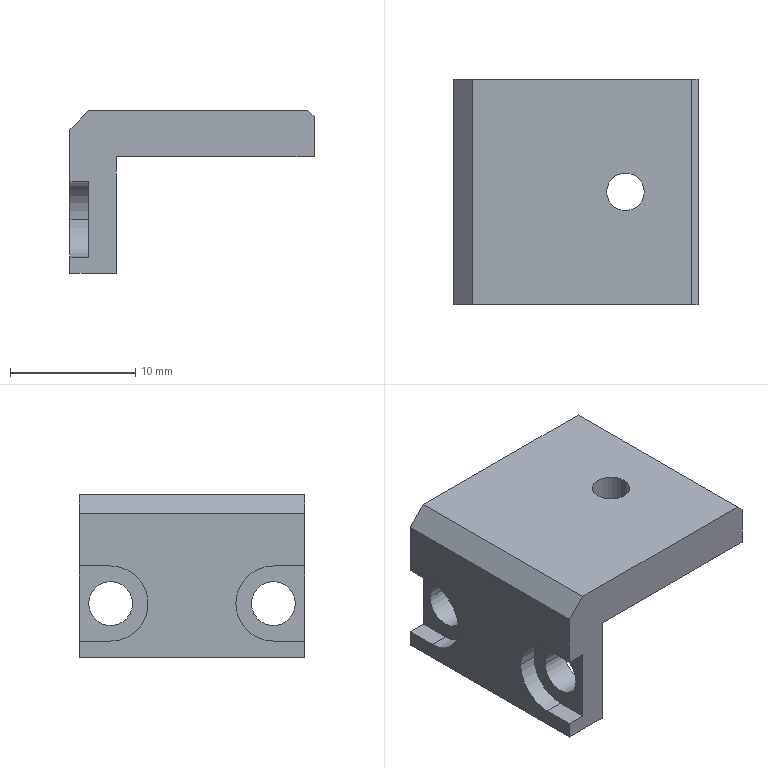Part | NX | 1 solid | 25 faces | box 19.5 x 18 x 13 mm | volume 1740 mm3 | plane 16 | cylinder 9 | commonest cylinder face diameters 3.5 x4 6 x3 3 x2
STEP:
#1=CARTESIAN_POINT('',(-5.3,9.,0.));
#2=VERTEX_POINT('',#1);
#3=CARTESIAN_POINT('',(-5.3,-9.,0.));
#4=VERTEX_POINT('',#3);
#5=CARTESIAN_POINT('',(-5.3,0.,0.));
#6=DIRECTION('',(0.,-1.,0.));
#7=VECTOR('',#6,1000.);
#8=LINE('',#5,#7);
#9=EDGE_CURVE('',#2,#4,#8,.T.);
#10=ORIENTED_EDGE('',*,*,#9,.T.);
#11=CARTESIAN_POINT('',(-9.,-9.,0.));
#12=VERTEX_POINT('',#11);
#13=CARTESIAN_POINT('',(0.,-9.,0.));
#14=DIRECTION('',(1.,0.,0.));
#15=VECTOR('',#14,1000.);
#16=LINE('',#13,#15);
#17=EDGE_CURVE('',#12,#4,#16,.T.);
#18=ORIENTED_EDGE('',*,*,#17,.F.);
#19=CARTESIAN_POINT('',(-9.,9.,0.));
#20=VERTEX_POINT('',#19);
#21=CARTESIAN_POINT('',(-9.,0.,0.));
#22=DIRECTION('',(0.,1.,0.));
#23=VECTOR('',#22,1000.);
#24=LINE('',#21,#23);
#25=EDGE_CURVE('',#12,#20,#24,.T.);
#26=ORIENTED_EDGE('',*,*,#25,.T.);
#27=CARTESIAN_POINT('',(0.,9.,0.));
#28=DIRECTION('',(-1.,0.,0.));
#29=VECTOR('',#28,1000.);
#30=LINE('',#27,#29);
#31=EDGE_CURVE('',#2,#20,#30,.T.);
#32=ORIENTED_EDGE('',*,*,#31,.F.);
#33=EDGE_LOOP('',(#10,#18,#26,#32));
#34=FACE_BOUND('',#33,.T.);
#35=CARTESIAN_POINT('',(0.,0.,0.));
#36=DIRECTION('',(0.,0.,1.));
#37=DIRECTION('',(1.,0.,0.));
#38=AXIS2_PLACEMENT_3D('',#35,#36,#37);
#39=PLANE('',#38);
#40=ADVANCED_FACE('',(#34),#39,.F.);
#41=CARTESIAN_POINT('',(-7.5,9.,1.3));
#42=VERTEX_POINT('',#41);
#43=CARTESIAN_POINT('',(-7.5,9.,7.3));
#44=VERTEX_POINT('',#43);
#45=CARTESIAN_POINT('',(-7.5,9.,0.));
#46=DIRECTION('',(0.,0.,1.));
#47=VECTOR('',#46,1000.);
#48=LINE('',#45,#47);
#49=EDGE_CURVE('',#42,#44,#48,.T.);
#50=ORIENTED_EDGE('',*,*,#49,.F.);
#51=CARTESIAN_POINT('',(-7.5,6.5,1.3));
#52=VERTEX_POINT('',#51);
#53=CARTESIAN_POINT('',(-7.5,0.,1.3));
#54=DIRECTION('',(0.,1.,0.));
#55=VECTOR('',#54,1000.);
#56=LINE('',#53,#55);
#57=EDGE_CURVE('',#52,#42,#56,.T.);
#58=ORIENTED_EDGE('',*,*,#57,.F.);
#59=CARTESIAN_POINT('',(-7.5,6.5,7.3));
#60=VERTEX_POINT('',#59);
#61=CARTESIAN_POINT('',(-7.5,6.5,4.3));
#62=DIRECTION('',(1.,0.,0.));
#63=DIRECTION('',(0.,1.,0.));
#64=AXIS2_PLACEMENT_3D('',#61,#62,#63);
#65=CIRCLE('',#64,3.);
#66=EDGE_CURVE('',#60,#52,#65,.T.);
#67=ORIENTED_EDGE('',*,*,#66,.F.);
#68=CARTESIAN_POINT('',(-7.5,0.,7.3));
#69=DIRECTION('',(0.,-1.,0.));
#70=VECTOR('',#69,1000.);
#71=LINE('',#68,#70);
#72=EDGE_CURVE('',#44,#60,#71,.T.);
#73=ORIENTED_EDGE('',*,*,#72,.F.);
#74=EDGE_LOOP('',(#50,#58,#67,#73));
#75=FACE_BOUND('',#74,.T.);
#76=CARTESIAN_POINT('',(-7.5,8.25,4.3));
#77=VERTEX_POINT('',#76);
#78=CARTESIAN_POINT('',(-7.5,4.75,4.3));
#79=VERTEX_POINT('',#78);
#80=CARTESIAN_POINT('',(-7.5,6.5,4.3));
#81=DIRECTION('',(1.,0.,0.));
#82=DIRECTION('',(0.,1.,0.));
#83=AXIS2_PLACEMENT_3D('',#80,#81,#82);
#84=CIRCLE('',#83,1.75);
#85=EDGE_CURVE('',#77,#79,#84,.T.);
#86=ORIENTED_EDGE('',*,*,#85,.T.);
#87=CARTESIAN_POINT('',(-7.5,6.5,4.3));
#88=DIRECTION('',(1.,0.,0.));
#89=DIRECTION('',(0.,1.,0.));
#90=AXIS2_PLACEMENT_3D('',#87,#88,#89);
#91=CIRCLE('',#90,1.75);
#92=EDGE_CURVE('',#79,#77,#91,.T.);
#93=ORIENTED_EDGE('',*,*,#92,.T.);
#94=EDGE_LOOP('',(#86,#93));
#95=FACE_BOUND('',#94,.T.);
#96=CARTESIAN_POINT('',(-7.5,6.5,4.3));
#97=DIRECTION('',(1.,0.,0.));
#98=DIRECTION('',(0.,1.,0.));
#99=AXIS2_PLACEMENT_3D('',#96,#97,#98);
#100=PLANE('',#99);
#101=ADVANCED_FACE('',(#75,#95),#100,.F.);
#102=CARTESIAN_POINT('',(10.5,-9.,12.5));
#103=VERTEX_POINT('',#102);
#104=CARTESIAN_POINT('',(10.5,-9.,9.3));
#105=VERTEX_POINT('',#104);
#106=CARTESIAN_POINT('',(10.5,-9.,0.));
#107=DIRECTION('',(0.,0.,-1.));
#108=VECTOR('',#107,1000.);
#109=LINE('',#106,#108);
#110=EDGE_CURVE('',#103,#105,#109,.T.);
#111=ORIENTED_EDGE('',*,*,#110,.F.);
#112=CARTESIAN_POINT('',(10.,-9.,13.));
#113=VERTEX_POINT('',#112);
#114=CARTESIAN_POINT('',(23.,-9.,0.));
#115=DIRECTION('',(0.7071,0.,-0.7071));
#116=VECTOR('',#115,1000.);
#117=LINE('',#114,#116);
#118=EDGE_CURVE('',#113,#103,#117,.T.);
#119=ORIENTED_EDGE('',*,*,#118,.F.);
#120=CARTESIAN_POINT('',(-7.5,-9.,13.));
#121=VERTEX_POINT('',#120);
#122=CARTESIAN_POINT('',(0.,-9.,13.));
#123=DIRECTION('',(1.,0.,0.));
#124=VECTOR('',#123,1000.);
#125=LINE('',#122,#124);
#126=EDGE_CURVE('',#121,#113,#125,.T.);
#127=ORIENTED_EDGE('',*,*,#126,.F.);
#128=CARTESIAN_POINT('',(-9.,-9.,11.5));
#129=VERTEX_POINT('',#128);
#130=CARTESIAN_POINT('',(-20.5,-9.,0.));
#131=DIRECTION('',(0.7071,0.,0.7071));
#132=VECTOR('',#131,1000.);
#133=LINE('',#130,#132);
#134=EDGE_CURVE('',#129,#121,#133,.T.);
#135=ORIENTED_EDGE('',*,*,#134,.F.);
#136=CARTESIAN_POINT('',(-9.,-9.,7.3));
#137=VERTEX_POINT('',#136);
#138=CARTESIAN_POINT('',(-9.,-9.,0.));
#139=DIRECTION('',(0.,0.,1.));
#140=VECTOR('',#139,1000.);
#141=LINE('',#138,#140);
#142=EDGE_CURVE('',#137,#129,#141,.T.);
#143=ORIENTED_EDGE('',*,*,#142,.F.);
#144=CARTESIAN_POINT('',(-7.5,-9.,7.3));
#145=VERTEX_POINT('',#144);
#146=CARTESIAN_POINT('',(0.,-9.,7.3));
#147=DIRECTION('',(1.,0.,0.));
#148=VECTOR('',#147,1000.);
#149=LINE('',#146,#148);
#150=EDGE_CURVE('',#137,#145,#149,.T.);
#151=ORIENTED_EDGE('',*,*,#150,.T.);
#152=CARTESIAN_POINT('',(-7.5,-9.,1.3));
#153=VERTEX_POINT('',#152);
#154=CARTESIAN_POINT('',(-7.5,-9.,0.));
#155=DIRECTION('',(0.,0.,-1.));
#156=VECTOR('',#155,1000.);
#157=LINE('',#154,#156);
#158=EDGE_CURVE('',#145,#153,#157,.T.);
#159=ORIENTED_EDGE('',*,*,#158,.T.);
#160=CARTESIAN_POINT('',(-9.,-9.,1.3));
#161=VERTEX_POINT('',#160);
#162=CARTESIAN_POINT('',(0.,-9.,1.3));
#163=DIRECTION('',(-1.,0.,0.));
#164=VECTOR('',#163,1000.);
#165=LINE('',#162,#164);
#166=EDGE_CURVE('',#153,#161,#165,.T.);
#167=ORIENTED_EDGE('',*,*,#166,.T.);
#168=CARTESIAN_POINT('',(-9.,-9.,0.));
#169=DIRECTION('',(0.,0.,1.));
#170=VECTOR('',#169,1000.);
#171=LINE('',#168,#170);
#172=EDGE_CURVE('',#12,#161,#171,.T.);
#173=ORIENTED_EDGE('',*,*,#172,.F.);
#174=ORIENTED_EDGE('',*,*,#17,.T.);
#175=CARTESIAN_POINT('',(-5.3,-9.,9.3));
#176=VERTEX_POINT('',#175);
#177=CARTESIAN_POINT('',(-5.3,-9.,0.));
#178=DIRECTION('',(0.,0.,-1.));
#179=VECTOR('',#178,1000.);
#180=LINE('',#177,#179);
#181=EDGE_CURVE('',#176,#4,#180,.T.);
#182=ORIENTED_EDGE('',*,*,#181,.F.);
#183=CARTESIAN_POINT('',(0.,-9.,9.3));
#184=DIRECTION('',(-1.,0.,0.));
#185=VECTOR('',#184,1000.);
#186=LINE('',#183,#185);
#187=EDGE_CURVE('',#105,#176,#186,.T.);
#188=ORIENTED_EDGE('',*,*,#187,.F.);
#189=EDGE_LOOP('',(#111,#119,#127,#135,#143,#151,#159,#167,#173,#174,#182,#188));
#190=FACE_BOUND('',#189,.T.);
#191=CARTESIAN_POINT('',(-10.5,-9.,0.));
#192=DIRECTION('',(0.,-1.,0.));
#193=DIRECTION('',(0.,0.,-1.));
#194=AXIS2_PLACEMENT_3D('',#191,#192,#193);
#195=PLANE('',#194);
#196=ADVANCED_FACE('',(#190),#195,.T.);
#197=ORIENTED_EDGE('',*,*,#158,.F.);
#198=CARTESIAN_POINT('',(-7.5,-6.5,7.3));
#199=VERTEX_POINT('',#198);
#200=CARTESIAN_POINT('',(-7.5,0.,7.3));
#201=DIRECTION('',(0.,-1.,0.));
#202=VECTOR('',#201,1000.);
#203=LINE('',#200,#202);
#204=EDGE_CURVE('',#199,#145,#203,.T.);
#205=ORIENTED_EDGE('',*,*,#204,.F.);
#206=CARTESIAN_POINT('',(-7.5,-3.5,4.3));
#207=VERTEX_POINT('',#206);
#208=CARTESIAN_POINT('',(-7.5,-6.5,4.3));
#209=DIRECTION('',(1.,0.,0.));
#210=DIRECTION('',(0.,1.,0.));
#211=AXIS2_PLACEMENT_3D('',#208,#209,#210);
#212=CIRCLE('',#211,3.);
#213=EDGE_CURVE('',#207,#199,#212,.T.);
#214=ORIENTED_EDGE('',*,*,#213,.F.);
#215=CARTESIAN_POINT('',(-7.5,-6.5,1.3));
#216=VERTEX_POINT('',#215);
#217=CARTESIAN_POINT('',(-7.5,-6.5,4.3));
#218=DIRECTION('',(1.,0.,0.));
#219=DIRECTION('',(0.,1.,0.));
#220=AXIS2_PLACEMENT_3D('',#217,#218,#219);
#221=CIRCLE('',#220,3.);
#222=EDGE_CURVE('',#216,#207,#221,.T.);
#223=ORIENTED_EDGE('',*,*,#222,.F.);
#224=CARTESIAN_POINT('',(-7.5,0.,1.3));
#225=DIRECTION('',(0.,1.,0.));
#226=VECTOR('',#225,1000.);
#227=LINE('',#224,#226);
#228=EDGE_CURVE('',#153,#216,#227,.T.);
#229=ORIENTED_EDGE('',*,*,#228,.F.);
#230=EDGE_LOOP('',(#197,#205,#214,#223,#229));
#231=FACE_BOUND('',#230,.T.);
#232=CARTESIAN_POINT('',(-7.5,-8.25,4.3));
#233=VERTEX_POINT('',#232);
#234=CARTESIAN_POINT('',(-7.5,-4.75,4.3));
#235=VERTEX_POINT('',#234);
#236=CARTESIAN_POINT('',(-7.5,-6.5,4.3));
#237=DIRECTION('',(1.,0.,0.));
#238=DIRECTION('',(0.,1.,0.));
#239=AXIS2_PLACEMENT_3D('',#236,#237,#238);
#240=CIRCLE('',#239,1.75);
#241=EDGE_CURVE('',#233,#235,#240,.T.);
#242=ORIENTED_EDGE('',*,*,#241,.T.);
#243=CARTESIAN_POINT('',(-7.5,-6.5,4.3));
#244=DIRECTION('',(1.,0.,0.));
#245=DIRECTION('',(0.,1.,0.));
#246=AXIS2_PLACEMENT_3D('',#243,#244,#245);
#247=CIRCLE('',#246,1.75);
#248=EDGE_CURVE('',#235,#233,#247,.T.);
#249=ORIENTED_EDGE('',*,*,#248,.T.);
#250=EDGE_LOOP('',(#242,#249));
#251=FACE_BOUND('',#250,.T.);
#252=CARTESIAN_POINT('',(-7.5,6.5,4.3));
#253=DIRECTION('',(1.,0.,0.));
#254=DIRECTION('',(0.,1.,0.));
#255=AXIS2_PLACEMENT_3D('',#252,#253,#254);
#256=PLANE('',#255);
#257=ADVANCED_FACE('',(#231,#251),#256,.F.);
#258=CARTESIAN_POINT('',(-9.,-6.5,1.3));
#259=VERTEX_POINT('',#258);
#260=CARTESIAN_POINT('',(-9.,0.,1.3));
#261=DIRECTION('',(0.,-1.,0.));
#262=VECTOR('',#261,1000.);
#263=LINE('',#260,#262);
#264=EDGE_CURVE('',#259,#161,#263,.T.);
#265=ORIENTED_EDGE('',*,*,#264,.T.);
#266=ORIENTED_EDGE('',*,*,#166,.F.);
#267=ORIENTED_EDGE('',*,*,#228,.T.);
#268=CARTESIAN_POINT('',(-7.5,-6.5,1.3));
#269=DIRECTION('',(-1.,0.,0.));
#270=VECTOR('',#269,1000.);
#271=LINE('',#268,#270);
#272=EDGE_CURVE('',#216,#259,#271,.T.);
#273=ORIENTED_EDGE('',*,*,#272,.T.);
#274=EDGE_LOOP('',(#265,#266,#267,#273));
#275=FACE_BOUND('',#274,.T.);
#276=CARTESIAN_POINT('',(-10.5,-6.5,1.3));
#277=DIRECTION('',(0.,0.,-1.));
#278=DIRECTION('',(0.,-1.,0.));
#279=AXIS2_PLACEMENT_3D('',#276,#277,#278);
#280=PLANE('',#279);
#281=ADVANCED_FACE('',(#275),#280,.F.);
#282=CARTESIAN_POINT('',(-9.,9.,11.5));
#283=VERTEX_POINT('',#282);
#284=CARTESIAN_POINT('',(-9.,0.,11.5));
#285=DIRECTION('',(0.,1.,0.));
#286=VECTOR('',#285,1000.);
#287=LINE('',#284,#286);
#288=EDGE_CURVE('',#129,#283,#287,.T.);
#289=ORIENTED_EDGE('',*,*,#288,.T.);
#290=CARTESIAN_POINT('',(-9.,9.,7.3));
#291=VERTEX_POINT('',#290);
#292=CARTESIAN_POINT('',(-9.,9.,0.));
#293=DIRECTION('',(0.,0.,-1.));
#294=VECTOR('',#293,1000.);
#295=LINE('',#292,#294);
#296=EDGE_CURVE('',#283,#291,#295,.T.);
#297=ORIENTED_EDGE('',*,*,#296,.T.);
#298=CARTESIAN_POINT('',(-9.,6.5,7.3));
#299=VERTEX_POINT('',#298);
#300=CARTESIAN_POINT('',(-9.,0.,7.3));
#301=DIRECTION('',(0.,1.,0.));
#302=VECTOR('',#301,1000.);
#303=LINE('',#300,#302);
#304=EDGE_CURVE('',#299,#291,#303,.T.);
#305=ORIENTED_EDGE('',*,*,#304,.F.);
#306=CARTESIAN_POINT('',(-9.,6.5,1.3));
#307=VERTEX_POINT('',#306);
#308=CARTESIAN_POINT('',(-9.,6.5,4.3));
#309=DIRECTION('',(1.,0.,0.));
#310=DIRECTION('',(0.,1.,0.));
#311=AXIS2_PLACEMENT_3D('',#308,#309,#310);
#312=CIRCLE('',#311,3.);
#313=EDGE_CURVE('',#299,#307,#312,.T.);
#314=ORIENTED_EDGE('',*,*,#313,.T.);
#315=CARTESIAN_POINT('',(-9.,9.,1.3));
#316=VERTEX_POINT('',#315);
#317=CARTESIAN_POINT('',(-9.,0.,1.3));
#318=DIRECTION('',(0.,-1.,0.));
#319=VECTOR('',#318,1000.);
#320=LINE('',#317,#319);
#321=EDGE_CURVE('',#316,#307,#320,.T.);
#322=ORIENTED_EDGE('',*,*,#321,.F.);
#323=CARTESIAN_POINT('',(-9.,9.,0.));
#324=DIRECTION('',(0.,0.,-1.));
#325=VECTOR('',#324,1000.);
#326=LINE('',#323,#325);
#327=EDGE_CURVE('',#316,#20,#326,.T.);
#328=ORIENTED_EDGE('',*,*,#327,.T.);
#329=ORIENTED_EDGE('',*,*,#25,.F.);
#330=ORIENTED_EDGE('',*,*,#172,.T.);
#331=ORIENTED_EDGE('',*,*,#264,.F.);
#332=CARTESIAN_POINT('',(-9.,-3.5,4.3));
#333=VERTEX_POINT('',#332);
#334=CARTESIAN_POINT('',(-9.,-6.5,4.3));
#335=DIRECTION('',(1.,0.,0.));
#336=DIRECTION('',(0.,1.,0.));
#337=AXIS2_PLACEMENT_3D('',#334,#335,#336);
#338=CIRCLE('',#337,3.);
#339=EDGE_CURVE('',#259,#333,#338,.T.);
#340=ORIENTED_EDGE('',*,*,#339,.T.);
#341=CARTESIAN_POINT('',(-9.,-6.5,7.3));
#342=VERTEX_POINT('',#341);
#343=CARTESIAN_POINT('',(-9.,-6.5,4.3));
#344=DIRECTION('',(1.,0.,0.));
#345=DIRECTION('',(0.,1.,0.));
#346=AXIS2_PLACEMENT_3D('',#343,#344,#345);
#347=CIRCLE('',#346,3.);
#348=EDGE_CURVE('',#333,#342,#347,.T.);
#349=ORIENTED_EDGE('',*,*,#348,.T.);
#350=CARTESIAN_POINT('',(-9.,0.,7.3));
#351=DIRECTION('',(0.,1.,0.));
#352=VECTOR('',#351,1000.);
#353=LINE('',#350,#352);
#354=EDGE_CURVE('',#137,#342,#353,.T.);
#355=ORIENTED_EDGE('',*,*,#354,.F.);
#356=ORIENTED_EDGE('',*,*,#142,.T.);
#357=EDGE_LOOP('',(#289,#297,#305,#314,#322,#328,#329,#330,#331,#340,#349,#355,#356));
#358=FACE_BOUND('',#357,.T.);
#359=CARTESIAN_POINT('',(-9.,9.,0.));
#360=DIRECTION('',(-1.,0.,0.));
#361=DIRECTION('',(0.,0.,1.));
#362=AXIS2_PLACEMENT_3D('',#359,#360,#361);
#363=PLANE('',#362);
#364=ADVANCED_FACE('',(#358),#363,.T.);
#365=ORIENTED_EDGE('',*,*,#321,.T.);
#366=CARTESIAN_POINT('',(-10.5,6.5,1.3));
#367=DIRECTION('',(1.,0.,0.));
#368=VECTOR('',#367,1000.);
#369=LINE('',#366,#368);
#370=EDGE_CURVE('',#307,#52,#369,.T.);
#371=ORIENTED_EDGE('',*,*,#370,.T.);
#372=ORIENTED_EDGE('',*,*,#57,.T.);
#373=CARTESIAN_POINT('',(0.,9.,1.3));
#374=DIRECTION('',(1.,0.,0.));
#375=VECTOR('',#374,1000.);
#376=LINE('',#373,#375);
#377=EDGE_CURVE('',#316,#42,#376,.T.);
#378=ORIENTED_EDGE('',*,*,#377,.F.);
#379=EDGE_LOOP('',(#365,#371,#372,#378));
#380=FACE_BOUND('',#379,.T.);
#381=CARTESIAN_POINT('',(-10.5,9.,1.3));
#382=DIRECTION('',(0.,0.,-1.));
#383=DIRECTION('',(0.,-1.,0.));
#384=AXIS2_PLACEMENT_3D('',#381,#382,#383);
#385=PLANE('',#384);
#386=ADVANCED_FACE('',(#380),#385,.F.);
#387=CARTESIAN_POINT('',(10.5,9.,9.3));
#388=VERTEX_POINT('',#387);
#389=CARTESIAN_POINT('',(-5.3,9.,9.3));
#390=VERTEX_POINT('',#389);
#391=CARTESIAN_POINT('',(0.,9.,9.3));
#392=DIRECTION('',(-1.,0.,0.));
#393=VECTOR('',#392,1000.);
#394=LINE('',#391,#393);
#395=EDGE_CURVE('',#388,#390,#394,.T.);
#396=ORIENTED_EDGE('',*,*,#395,.T.);
#397=CARTESIAN_POINT('',(-5.3,9.,0.));
#398=DIRECTION('',(0.,0.,-1.));
#399=VECTOR('',#398,1000.);
#400=LINE('',#397,#399);
#401=EDGE_CURVE('',#390,#2,#400,.T.);
#402=ORIENTED_EDGE('',*,*,#401,.T.);
#403=ORIENTED_EDGE('',*,*,#31,.T.);
#404=ORIENTED_EDGE('',*,*,#327,.F.);
#405=ORIENTED_EDGE('',*,*,#377,.T.);
#406=ORIENTED_EDGE('',*,*,#49,.T.);
#407=CARTESIAN_POINT('',(0.,9.,7.3));
#408=DIRECTION('',(-1.,0.,0.));
#409=VECTOR('',#408,1000.);
#410=LINE('',#407,#409);
#411=EDGE_CURVE('',#44,#291,#410,.T.);
#412=ORIENTED_EDGE('',*,*,#411,.T.);
#413=ORIENTED_EDGE('',*,*,#296,.F.);
#414=CARTESIAN_POINT('',(-7.5,9.,13.));
#415=VERTEX_POINT('',#414);
#416=CARTESIAN_POINT('',(-20.5,9.,0.));
#417=DIRECTION('',(-0.7071,0.,-0.7071));
#418=VECTOR('',#417,1000.);
#419=LINE('',#416,#418);
#420=EDGE_CURVE('',#415,#283,#419,.T.);
#421=ORIENTED_EDGE('',*,*,#420,.F.);
#422=CARTESIAN_POINT('',(10.,9.,13.));
#423=VERTEX_POINT('',#422);
#424=CARTESIAN_POINT('',(0.,9.,13.));
#425=DIRECTION('',(-1.,0.,0.));
#426=VECTOR('',#425,1000.);
#427=LINE('',#424,#426);
#428=EDGE_CURVE('',#423,#415,#427,.T.);
#429=ORIENTED_EDGE('',*,*,#428,.F.);
#430=CARTESIAN_POINT('',(10.5,9.,12.5));
#431=VERTEX_POINT('',#430);
#432=CARTESIAN_POINT('',(23.,9.,0.));
#433=DIRECTION('',(-0.7071,0.,0.7071));
#434=VECTOR('',#433,1000.);
#435=LINE('',#432,#434);
#436=EDGE_CURVE('',#431,#423,#435,.T.);
#437=ORIENTED_EDGE('',*,*,#436,.F.);
#438=CARTESIAN_POINT('',(10.5,9.,0.));
#439=DIRECTION('',(0.,0.,1.));
#440=VECTOR('',#439,1000.);
#441=LINE('',#438,#440);
#442=EDGE_CURVE('',#388,#431,#441,.T.);
#443=ORIENTED_EDGE('',*,*,#442,.F.);
#444=EDGE_LOOP('',(#396,#402,#403,#404,#405,#406,#412,#413,#421,#429,#437,#443));
#445=FACE_BOUND('',#444,.T.);
#446=CARTESIAN_POINT('',(10.5,9.,0.));
#447=DIRECTION('',(0.,1.,0.));
#448=DIRECTION('',(1.,0.,0.));
#449=AXIS2_PLACEMENT_3D('',#446,#447,#448);
#450=PLANE('',#449);
#451=ADVANCED_FACE('',(#445),#450,.T.);
#452=CARTESIAN_POINT('',(-7.5,0.,13.));
#453=DIRECTION('',(0.,1.,0.));
#454=VECTOR('',#453,1000.);
#455=LINE('',#452,#454);
#456=EDGE_CURVE('',#121,#415,#455,.T.);
#457=ORIENTED_EDGE('',*,*,#456,.F.);
#458=ORIENTED_EDGE('',*,*,#126,.T.);
#459=CARTESIAN_POINT('',(10.,0.,13.));
#460=DIRECTION('',(0.,-1.,0.));
#461=VECTOR('',#460,1000.);
#462=LINE('',#459,#461);
#463=EDGE_CURVE('',#423,#113,#462,.T.);
#464=ORIENTED_EDGE('',*,*,#463,.F.);
#465=ORIENTED_EDGE('',*,*,#428,.T.);
#466=EDGE_LOOP('',(#457,#458,#464,#465));
#467=FACE_BOUND('',#466,.T.);
#468=CARTESIAN_POINT('',(6.2,0.,13.));
#469=VERTEX_POINT('',#468);
#470=CARTESIAN_POINT('',(3.2,0.,13.));
#471=VERTEX_POINT('',#470);
#472=CARTESIAN_POINT('',(4.7,0.,13.));
#473=DIRECTION('',(0.,0.,-1.));
#474=DIRECTION('',(-1.,0.,0.));
#475=AXIS2_PLACEMENT_3D('',#472,#473,#474);
#476=CIRCLE('',#475,1.5);
#477=EDGE_CURVE('',#469,#471,#476,.T.);
#478=ORIENTED_EDGE('',*,*,#477,.T.);
#479=CARTESIAN_POINT('',(4.7,0.,13.));
#480=DIRECTION('',(0.,0.,-1.));
#481=DIRECTION('',(-1.,0.,0.));
#482=AXIS2_PLACEMENT_3D('',#479,#480,#481);
#483=CIRCLE('',#482,1.5);
#484=EDGE_CURVE('',#471,#469,#483,.T.);
#485=ORIENTED_EDGE('',*,*,#484,.T.);
#486=EDGE_LOOP('',(#478,#485));
#487=FACE_BOUND('',#486,.T.);
#488=CARTESIAN_POINT('',(0.,0.,13.));
#489=DIRECTION('',(0.,0.,1.));
#490=DIRECTION('',(1.,0.,0.));
#491=AXIS2_PLACEMENT_3D('',#488,#489,#490);
#492=PLANE('',#491);
#493=ADVANCED_FACE('',(#467,#487),#492,.T.);
#494=ORIENTED_EDGE('',*,*,#304,.T.);
#495=ORIENTED_EDGE('',*,*,#411,.F.);
#496=ORIENTED_EDGE('',*,*,#72,.T.);
#497=CARTESIAN_POINT('',(-7.5,6.5,7.3));
#498=DIRECTION('',(-1.,0.,0.));
#499=VECTOR('',#498,1000.);
#500=LINE('',#497,#499);
#501=EDGE_CURVE('',#60,#299,#500,.T.);
#502=ORIENTED_EDGE('',*,*,#501,.T.);
#503=EDGE_LOOP('',(#494,#495,#496,#502));
#504=FACE_BOUND('',#503,.T.);
#505=CARTESIAN_POINT('',(-10.5,6.5,7.3));
#506=DIRECTION('',(0.,0.,1.));
#507=DIRECTION('',(1.,0.,0.));
#508=AXIS2_PLACEMENT_3D('',#505,#506,#507);
#509=PLANE('',#508);
#510=ADVANCED_FACE('',(#504),#509,.F.);
#511=ORIENTED_EDGE('',*,*,#370,.F.);
#512=ORIENTED_EDGE('',*,*,#313,.F.);
#513=ORIENTED_EDGE('',*,*,#501,.F.);
#514=ORIENTED_EDGE('',*,*,#66,.T.);
#515=EDGE_LOOP('',(#511,#512,#513,#514));
#516=FACE_BOUND('',#515,.T.);
#517=CARTESIAN_POINT('',(-10.5,6.5,4.3));
#518=DIRECTION('',(1.,0.,0.));
#519=DIRECTION('',(0.,1.,0.));
#520=AXIS2_PLACEMENT_3D('',#517,#518,#519);
#521=CYLINDRICAL_SURFACE('',#520,3.);
#522=ADVANCED_FACE('',(#516),#521,.F.);
#523=CARTESIAN_POINT('',(-5.3,4.75,4.3));
#524=VERTEX_POINT('',#523);
#525=CARTESIAN_POINT('',(-5.3,8.25,4.3));
#526=VERTEX_POINT('',#525);
#527=CARTESIAN_POINT('',(-5.3,6.5,4.3));
#528=DIRECTION('',(1.,0.,0.));
#529=DIRECTION('',(0.,1.,0.));
#530=AXIS2_PLACEMENT_3D('',#527,#528,#529);
#531=CIRCLE('',#530,1.75);
#532=EDGE_CURVE('',#524,#526,#531,.T.);
#533=ORIENTED_EDGE('',*,*,#532,.T.);
#534=CARTESIAN_POINT('',(-10.5,8.25,4.3));
#535=DIRECTION('',(1.,0.,0.));
#536=VECTOR('',#535,1000.);
#537=LINE('',#534,#536);
#538=EDGE_CURVE('',#77,#526,#537,.T.);
#539=ORIENTED_EDGE('',*,*,#538,.F.);
#540=ORIENTED_EDGE('',*,*,#92,.F.);
#541=CARTESIAN_POINT('',(-10.5,4.75,4.3));
#542=DIRECTION('',(1.,0.,0.));
#543=VECTOR('',#542,1000.);
#544=LINE('',#541,#543);
#545=EDGE_CURVE('',#79,#524,#544,.T.);
#546=ORIENTED_EDGE('',*,*,#545,.T.);
#547=EDGE_LOOP('',(#533,#539,#540,#546));
#548=FACE_BOUND('',#547,.T.);
#549=CARTESIAN_POINT('',(-10.5,6.5,4.3));
#550=DIRECTION('',(1.,0.,0.));
#551=DIRECTION('',(0.,1.,0.));
#552=AXIS2_PLACEMENT_3D('',#549,#550,#551);
#553=CYLINDRICAL_SURFACE('',#552,1.75);
#554=ADVANCED_FACE('',(#548),#553,.F.);
#555=CARTESIAN_POINT('',(-10.5,-3.5,4.3));
#556=DIRECTION('',(1.,0.,0.));
#557=VECTOR('',#556,1000.);
#558=LINE('',#555,#557);
#559=EDGE_CURVE('',#333,#207,#558,.T.);
#560=ORIENTED_EDGE('',*,*,#559,.F.);
#561=ORIENTED_EDGE('',*,*,#339,.F.);
#562=ORIENTED_EDGE('',*,*,#272,.F.);
#563=ORIENTED_EDGE('',*,*,#222,.T.);
#564=EDGE_LOOP('',(#560,#561,#562,#563));
#565=FACE_BOUND('',#564,.T.);
#566=CARTESIAN_POINT('',(-10.5,-6.5,4.3));
#567=DIRECTION('',(1.,0.,0.));
#568=DIRECTION('',(0.,1.,0.));
#569=AXIS2_PLACEMENT_3D('',#566,#567,#568);
#570=CYLINDRICAL_SURFACE('',#569,3.);
#571=ADVANCED_FACE('',(#565),#570,.F.);
#572=ORIENTED_EDGE('',*,*,#9,.F.);
#573=ORIENTED_EDGE('',*,*,#401,.F.);
#574=CARTESIAN_POINT('',(-5.3,0.,9.3));
#575=DIRECTION('',(0.,-1.,0.));
#576=VECTOR('',#575,1000.);
#577=LINE('',#574,#576);
#578=EDGE_CURVE('',#390,#176,#577,.T.);
#579=ORIENTED_EDGE('',*,*,#578,.T.);
#580=ORIENTED_EDGE('',*,*,#181,.T.);
#581=EDGE_LOOP('',(#572,#573,#579,#580));
#582=FACE_BOUND('',#581,.T.);
#583=ORIENTED_EDGE('',*,*,#532,.F.);
#584=CARTESIAN_POINT('',(-5.3,6.5,4.3));
#585=DIRECTION('',(1.,0.,0.));
#586=DIRECTION('',(0.,1.,0.));
#587=AXIS2_PLACEMENT_3D('',#584,#585,#586);
#588=CIRCLE('',#587,1.75);
#589=EDGE_CURVE('',#526,#524,#588,.T.);
#590=ORIENTED_EDGE('',*,*,#589,.F.);
#591=EDGE_LOOP('',(#583,#590));
#592=FACE_BOUND('',#591,.T.);
#593=CARTESIAN_POINT('',(-5.3,-4.75,4.3));
#594=VERTEX_POINT('',#593);
#595=CARTESIAN_POINT('',(-5.3,-8.25,4.3));
#596=VERTEX_POINT('',#595);
#597=CARTESIAN_POINT('',(-5.3,-6.5,4.3));
#598=DIRECTION('',(1.,0.,0.));
#599=DIRECTION('',(0.,1.,0.));
#600=AXIS2_PLACEMENT_3D('',#597,#598,#599);
#601=CIRCLE('',#600,1.75);
#602=EDGE_CURVE('',#594,#596,#601,.T.);
#603=ORIENTED_EDGE('',*,*,#602,.F.);
#604=CARTESIAN_POINT('',(-5.3,-6.5,4.3));
#605=DIRECTION('',(1.,0.,0.));
#606=DIRECTION('',(0.,1.,0.));
#607=AXIS2_PLACEMENT_3D('',#604,#605,#606);
#608=CIRCLE('',#607,1.75);
#609=EDGE_CURVE('',#596,#594,#608,.T.);
#610=ORIENTED_EDGE('',*,*,#609,.F.);
#611=EDGE_LOOP('',(#603,#610));
#612=FACE_BOUND('',#611,.T.);
#613=CARTESIAN_POINT('',(-5.3,-9.,9.3));
#614=DIRECTION('',(-1.,0.,0.));
#615=DIRECTION('',(0.,0.,1.));
#616=AXIS2_PLACEMENT_3D('',#613,#614,#615);
#617=PLANE('',#616);
#618=ADVANCED_FACE('',(#582,#592,#612),#617,.F.);
#619=CARTESIAN_POINT('',(10.5,0.,9.3));
#620=DIRECTION('',(0.,-1.,0.));
#621=VECTOR('',#620,1000.);
#622=LINE('',#619,#621);
#623=EDGE_CURVE('',#388,#105,#622,.T.);
#624=ORIENTED_EDGE('',*,*,#623,.F.);
#625=ORIENTED_EDGE('',*,*,#442,.T.);
#626=CARTESIAN_POINT('',(10.5,0.,12.5));
#627=DIRECTION('',(0.,1.,0.));
#628=VECTOR('',#627,1000.);
#629=LINE('',#626,#628);
#630=EDGE_CURVE('',#103,#431,#629,.T.);
#631=ORIENTED_EDGE('',*,*,#630,.F.);
#632=ORIENTED_EDGE('',*,*,#110,.T.);
#633=EDGE_LOOP('',(#624,#625,#631,#632));
#634=FACE_BOUND('',#633,.T.);
#635=CARTESIAN_POINT('',(10.5,-9.,0.));
#636=DIRECTION('',(1.,0.,0.));
#637=DIRECTION('',(0.,1.,0.));
#638=AXIS2_PLACEMENT_3D('',#635,#636,#637);
#639=PLANE('',#638);
#640=ADVANCED_FACE('',(#634),#639,.T.);
#641=ORIENTED_EDGE('',*,*,#623,.T.);
#642=ORIENTED_EDGE('',*,*,#187,.T.);
#643=ORIENTED_EDGE('',*,*,#578,.F.);
#644=ORIENTED_EDGE('',*,*,#395,.F.);
#645=EDGE_LOOP('',(#641,#642,#643,#644));
#646=FACE_BOUND('',#645,.T.);
#647=CARTESIAN_POINT('',(3.2,0.,9.3));
#648=VERTEX_POINT('',#647);
#649=CARTESIAN_POINT('',(6.2,0.,9.3));
#650=VERTEX_POINT('',#649);
#651=CARTESIAN_POINT('',(4.7,0.,9.3));
#652=DIRECTION('',(0.,0.,-1.));
#653=DIRECTION('',(-1.,0.,0.));
#654=AXIS2_PLACEMENT_3D('',#651,#652,#653);
#655=CIRCLE('',#654,1.5);
#656=EDGE_CURVE('',#648,#650,#655,.T.);
#657=ORIENTED_EDGE('',*,*,#656,.F.);
#658=CARTESIAN_POINT('',(4.7,0.,9.3));
#659=DIRECTION('',(0.,0.,-1.));
#660=DIRECTION('',(-1.,0.,0.));
#661=AXIS2_PLACEMENT_3D('',#658,#659,#660);
#662=CIRCLE('',#661,1.5);
#663=EDGE_CURVE('',#650,#648,#662,.T.);
#664=ORIENTED_EDGE('',*,*,#663,.F.);
#665=EDGE_LOOP('',(#657,#664));
#666=FACE_BOUND('',#665,.T.);
#667=CARTESIAN_POINT('',(10.5,-9.,9.3));
#668=DIRECTION('',(0.,0.,1.));
#669=DIRECTION('',(1.,0.,0.));
#670=AXIS2_PLACEMENT_3D('',#667,#668,#669);
#671=PLANE('',#670);
#672=ADVANCED_FACE('',(#646,#666),#671,.F.);
#673=ORIENTED_EDGE('',*,*,#630,.T.);
#674=ORIENTED_EDGE('',*,*,#436,.T.);
#675=ORIENTED_EDGE('',*,*,#463,.T.);
#676=ORIENTED_EDGE('',*,*,#118,.T.);
#677=EDGE_LOOP('',(#673,#674,#675,#676));
#678=FACE_BOUND('',#677,.T.);
#679=CARTESIAN_POINT('',(10.25,0.,12.75));
#680=DIRECTION('',(0.7071,0.,0.7071));
#681=DIRECTION('',(0.,-1.,0.));
#682=AXIS2_PLACEMENT_3D('',#679,#680,#681);
#683=PLANE('',#682);
#684=ADVANCED_FACE('',(#678),#683,.T.);
#685=ORIENTED_EDGE('',*,*,#602,.T.);
#686=CARTESIAN_POINT('',(-10.5,-8.25,4.3));
#687=DIRECTION('',(1.,0.,0.));
#688=VECTOR('',#687,1000.);
#689=LINE('',#686,#688);
#690=EDGE_CURVE('',#596,#233,#689,.F.);
#691=ORIENTED_EDGE('',*,*,#690,.T.);
#692=ORIENTED_EDGE('',*,*,#248,.F.);
#693=CARTESIAN_POINT('',(-10.5,-4.75,4.3));
#694=DIRECTION('',(1.,0.,0.));
#695=VECTOR('',#694,1000.);
#696=LINE('',#693,#695);
#697=EDGE_CURVE('',#594,#235,#696,.F.);
#698=ORIENTED_EDGE('',*,*,#697,.F.);
#699=EDGE_LOOP('',(#685,#691,#692,#698));
#700=FACE_BOUND('',#699,.T.);
#701=CARTESIAN_POINT('',(-10.5,-6.5,4.3));
#702=DIRECTION('',(1.,0.,0.));
#703=DIRECTION('',(0.,1.,0.));
#704=AXIS2_PLACEMENT_3D('',#701,#702,#703);
#705=CYLINDRICAL_SURFACE('',#704,1.75);
#706=ADVANCED_FACE('',(#700),#705,.F.);
#707=ORIENTED_EDGE('',*,*,#354,.T.);
#708=CARTESIAN_POINT('',(-10.5,-6.5,7.3));
#709=DIRECTION('',(1.,0.,0.));
#710=VECTOR('',#709,1000.);
#711=LINE('',#708,#710);
#712=EDGE_CURVE('',#342,#199,#711,.T.);
#713=ORIENTED_EDGE('',*,*,#712,.T.);
#714=ORIENTED_EDGE('',*,*,#204,.T.);
#715=ORIENTED_EDGE('',*,*,#150,.F.);
#716=EDGE_LOOP('',(#707,#713,#714,#715));
#717=FACE_BOUND('',#716,.T.);
#718=CARTESIAN_POINT('',(-10.5,-9.,7.3));
#719=DIRECTION('',(0.,0.,1.));
#720=DIRECTION('',(1.,0.,0.));
#721=AXIS2_PLACEMENT_3D('',#718,#719,#720);
#722=PLANE('',#721);
#723=ADVANCED_FACE('',(#717),#722,.F.);
#724=ORIENTED_EDGE('',*,*,#288,.F.);
#725=ORIENTED_EDGE('',*,*,#134,.T.);
#726=ORIENTED_EDGE('',*,*,#456,.T.);
#727=ORIENTED_EDGE('',*,*,#420,.T.);
#728=EDGE_LOOP('',(#724,#725,#726,#727));
#729=FACE_BOUND('',#728,.T.);
#730=CARTESIAN_POINT('',(-8.25,0.,12.25));
#731=DIRECTION('',(-0.7071,0.,0.7071));
#732=DIRECTION('',(0.,1.,0.));
#733=AXIS2_PLACEMENT_3D('',#730,#731,#732);
#734=PLANE('',#733);
#735=ADVANCED_FACE('',(#729),#734,.T.);
#736=ORIENTED_EDGE('',*,*,#477,.F.);
#737=CARTESIAN_POINT('',(6.2,0.,13.));
#738=DIRECTION('',(0.,0.,-1.));
#739=VECTOR('',#738,1000.);
#740=LINE('',#737,#739);
#741=EDGE_CURVE('',#469,#650,#740,.T.);
#742=ORIENTED_EDGE('',*,*,#741,.T.);
#743=ORIENTED_EDGE('',*,*,#663,.T.);
#744=CARTESIAN_POINT('',(3.2,0.,13.));
#745=DIRECTION('',(0.,0.,-1.));
#746=VECTOR('',#745,1000.);
#747=LINE('',#744,#746);
#748=EDGE_CURVE('',#471,#648,#747,.T.);
#749=ORIENTED_EDGE('',*,*,#748,.F.);
#750=EDGE_LOOP('',(#736,#742,#743,#749));
#751=FACE_BOUND('',#750,.T.);
#752=CARTESIAN_POINT('',(4.7,0.,13.));
#753=DIRECTION('',(0.,0.,-1.));
#754=DIRECTION('',(-1.,0.,0.));
#755=AXIS2_PLACEMENT_3D('',#752,#753,#754);
#756=CYLINDRICAL_SURFACE('',#755,1.5);
#757=ADVANCED_FACE('',(#751),#756,.F.);
#758=ORIENTED_EDGE('',*,*,#241,.F.);
#759=ORIENTED_EDGE('',*,*,#690,.F.);
#760=ORIENTED_EDGE('',*,*,#609,.T.);
#761=ORIENTED_EDGE('',*,*,#697,.T.);
#762=EDGE_LOOP('',(#758,#759,#760,#761));
#763=FACE_BOUND('',#762,.T.);
#764=CARTESIAN_POINT('',(-10.5,-6.5,4.3));
#765=DIRECTION('',(1.,0.,0.));
#766=DIRECTION('',(0.,1.,0.));
#767=AXIS2_PLACEMENT_3D('',#764,#765,#766);
#768=CYLINDRICAL_SURFACE('',#767,1.75);
#769=ADVANCED_FACE('',(#763),#768,.F.);
#770=ORIENTED_EDGE('',*,*,#85,.F.);
#771=ORIENTED_EDGE('',*,*,#538,.T.);
#772=ORIENTED_EDGE('',*,*,#589,.T.);
#773=ORIENTED_EDGE('',*,*,#545,.F.);
#774=EDGE_LOOP('',(#770,#771,#772,#773));
#775=FACE_BOUND('',#774,.T.);
#776=CARTESIAN_POINT('',(-10.5,6.5,4.3));
#777=DIRECTION('',(1.,0.,0.));
#778=DIRECTION('',(0.,1.,0.));
#779=AXIS2_PLACEMENT_3D('',#776,#777,#778);
#780=CYLINDRICAL_SURFACE('',#779,1.75);
#781=ADVANCED_FACE('',(#775),#780,.F.);
#782=ORIENTED_EDGE('',*,*,#656,.T.);
#783=ORIENTED_EDGE('',*,*,#741,.F.);
#784=ORIENTED_EDGE('',*,*,#484,.F.);
#785=ORIENTED_EDGE('',*,*,#748,.T.);
#786=EDGE_LOOP('',(#782,#783,#784,#785));
#787=FACE_BOUND('',#786,.T.);
#788=CARTESIAN_POINT('',(4.7,0.,13.));
#789=DIRECTION('',(0.,0.,-1.));
#790=DIRECTION('',(-1.,0.,0.));
#791=AXIS2_PLACEMENT_3D('',#788,#789,#790);
#792=CYLINDRICAL_SURFACE('',#791,1.5);
#793=ADVANCED_FACE('',(#787),#792,.F.);
#794=ORIENTED_EDGE('',*,*,#348,.F.);
#795=ORIENTED_EDGE('',*,*,#559,.T.);
#796=ORIENTED_EDGE('',*,*,#213,.T.);
#797=ORIENTED_EDGE('',*,*,#712,.F.);
#798=EDGE_LOOP('',(#794,#795,#796,#797));
#799=FACE_BOUND('',#798,.T.);
#800=CARTESIAN_POINT('',(-10.5,-6.5,4.3));
#801=DIRECTION('',(1.,0.,0.));
#802=DIRECTION('',(0.,1.,0.));
#803=AXIS2_PLACEMENT_3D('',#800,#801,#802);
#804=CYLINDRICAL_SURFACE('',#803,3.);
#805=ADVANCED_FACE('',(#799),#804,.F.);
#806=CLOSED_SHELL('',(#40,#101,#196,#257,#281,#364,#386,#451,#493,#510,#522,#554,#571,#618,#640,#672,#684,#706,#723,#735,#757,#769,#781,#793,#805));
#807=MANIFOLD_SOLID_BREP('',#806);
#808=(LENGTH_UNIT()NAMED_UNIT(*)SI_UNIT(.MILLI.,.METRE.));
#809=UNCERTAINTY_MEASURE_WITH_UNIT(LENGTH_MEASURE(0.00001),#808,'','');
#810=(NAMED_UNIT(*)PLANE_ANGLE_UNIT()SI_UNIT($,.RADIAN.));
#811=(NAMED_UNIT(*)SI_UNIT($,.STERADIAN.)SOLID_ANGLE_UNIT());
#812=(GEOMETRIC_REPRESENTATION_CONTEXT(3)GLOBAL_UNCERTAINTY_ASSIGNED_CONTEXT((#809))GLOBAL_UNIT_ASSIGNED_CONTEXT((#808,#810,#811))REPRESENTATION_CONTEXT('',''));
#813=ADVANCED_BREP_SHAPE_REPRESENTATION('',(#807),#812);